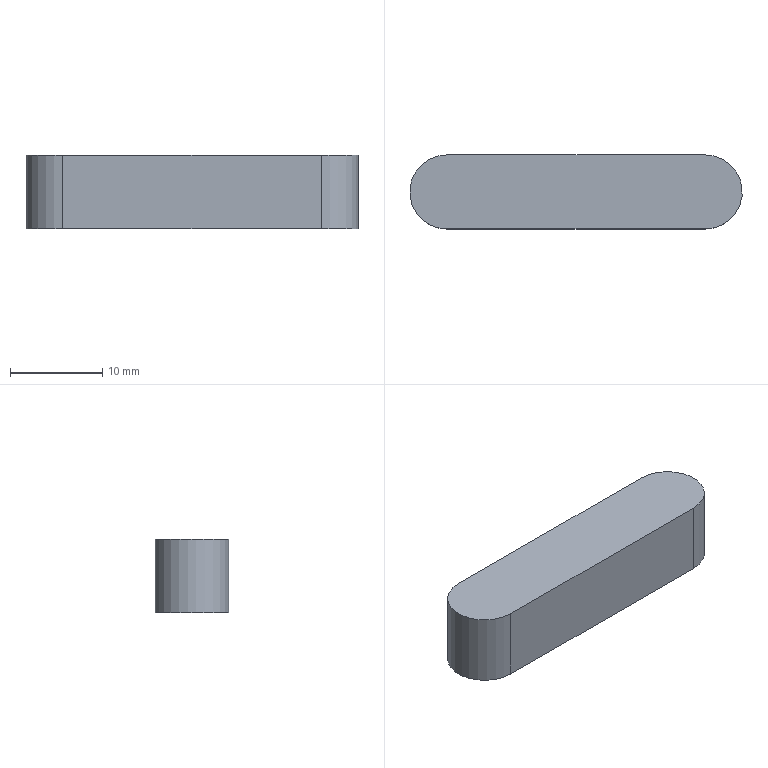Part | NX | features DATUM_CSYS 2, EXTRUDE 1, SKETCH 1 | 1 solid | 6 faces | box 36 x 8 x 8 mm | volume 2194 mm3 | plane 4 | cylinder 2 | commonest cylinder face diameters 8 x2
STEP:
#1=CARTESIAN_POINT('',(14.,-4.,0.));
#2=VERTEX_POINT('',#1);
#3=CARTESIAN_POINT('',(14.,4.,0.));
#4=VERTEX_POINT('',#3);
#5=CARTESIAN_POINT('',(14.,0.,0.));
#6=DIRECTION('',(0.,0.,1.));
#7=DIRECTION('',(-1.,0.,0.));
#8=AXIS2_PLACEMENT_3D('',#5,#6,#7);
#9=CIRCLE('',#8,4.);
#10=EDGE_CURVE('',#2,#4,#9,.T.);
#11=ORIENTED_EDGE('',*,*,#10,.T.);
#12=CARTESIAN_POINT('',(14.,4.,8.));
#13=VERTEX_POINT('',#12);
#14=CARTESIAN_POINT('',(14.,4.,8.));
#15=DIRECTION('',(0.,0.,-1.));
#16=VECTOR('',#15,1000.);
#17=LINE('',#14,#16);
#18=EDGE_CURVE('',#13,#4,#17,.T.);
#19=ORIENTED_EDGE('',*,*,#18,.F.);
#20=CARTESIAN_POINT('',(14.,-4.,8.));
#21=VERTEX_POINT('',#20);
#22=CARTESIAN_POINT('',(14.,0.,8.));
#23=DIRECTION('',(0.,0.,1.));
#24=DIRECTION('',(-1.,0.,0.));
#25=AXIS2_PLACEMENT_3D('',#22,#23,#24);
#26=CIRCLE('',#25,4.);
#27=EDGE_CURVE('',#21,#13,#26,.T.);
#28=ORIENTED_EDGE('',*,*,#27,.F.);
#29=CARTESIAN_POINT('',(14.,-4.,8.));
#30=DIRECTION('',(0.,0.,-1.));
#31=VECTOR('',#30,1000.);
#32=LINE('',#29,#31);
#33=EDGE_CURVE('',#21,#2,#32,.T.);
#34=ORIENTED_EDGE('',*,*,#33,.T.);
#35=EDGE_LOOP('',(#11,#19,#28,#34));
#36=FACE_BOUND('',#35,.T.);
#37=CARTESIAN_POINT('',(14.,0.,8.));
#38=DIRECTION('',(0.,0.,-1.));
#39=DIRECTION('',(-1.,0.,0.));
#40=AXIS2_PLACEMENT_3D('',#37,#38,#39);
#41=CYLINDRICAL_SURFACE('',#40,4.);
#42=ADVANCED_FACE('',(#36),#41,.T.);
#43=CARTESIAN_POINT('',(-14.,4.,0.));
#44=VERTEX_POINT('',#43);
#45=CARTESIAN_POINT('',(14.,4.,0.));
#46=DIRECTION('',(-1.,0.,0.));
#47=VECTOR('',#46,1000.);
#48=LINE('',#45,#47);
#49=EDGE_CURVE('',#4,#44,#48,.T.);
#50=ORIENTED_EDGE('',*,*,#49,.T.);
#51=CARTESIAN_POINT('',(-14.,4.,8.));
#52=VERTEX_POINT('',#51);
#53=CARTESIAN_POINT('',(-14.,4.,8.));
#54=DIRECTION('',(0.,0.,-1.));
#55=VECTOR('',#54,1000.);
#56=LINE('',#53,#55);
#57=EDGE_CURVE('',#52,#44,#56,.T.);
#58=ORIENTED_EDGE('',*,*,#57,.F.);
#59=CARTESIAN_POINT('',(14.,4.,8.));
#60=DIRECTION('',(-1.,0.,0.));
#61=VECTOR('',#60,1000.);
#62=LINE('',#59,#61);
#63=EDGE_CURVE('',#13,#52,#62,.T.);
#64=ORIENTED_EDGE('',*,*,#63,.F.);
#65=ORIENTED_EDGE('',*,*,#18,.T.);
#66=EDGE_LOOP('',(#50,#58,#64,#65));
#67=FACE_BOUND('',#66,.T.);
#68=CARTESIAN_POINT('',(14.,4.,8.));
#69=DIRECTION('',(0.,-1.,0.));
#70=DIRECTION('',(0.,0.,-1.));
#71=AXIS2_PLACEMENT_3D('',#68,#69,#70);
#72=PLANE('',#71);
#73=ADVANCED_FACE('',(#67),#72,.F.);
#74=CARTESIAN_POINT('',(-14.,-4.,0.));
#75=VERTEX_POINT('',#74);
#76=CARTESIAN_POINT('',(-14.,0.,0.));
#77=DIRECTION('',(0.,0.,1.));
#78=DIRECTION('',(1.,0.,0.));
#79=AXIS2_PLACEMENT_3D('',#76,#77,#78);
#80=CIRCLE('',#79,4.);
#81=EDGE_CURVE('',#44,#75,#80,.T.);
#82=ORIENTED_EDGE('',*,*,#81,.T.);
#83=CARTESIAN_POINT('',(-14.,-4.,8.));
#84=VERTEX_POINT('',#83);
#85=CARTESIAN_POINT('',(-14.,-4.,8.));
#86=DIRECTION('',(0.,0.,-1.));
#87=VECTOR('',#86,1000.);
#88=LINE('',#85,#87);
#89=EDGE_CURVE('',#84,#75,#88,.T.);
#90=ORIENTED_EDGE('',*,*,#89,.F.);
#91=CARTESIAN_POINT('',(-14.,0.,8.));
#92=DIRECTION('',(0.,0.,1.));
#93=DIRECTION('',(1.,0.,0.));
#94=AXIS2_PLACEMENT_3D('',#91,#92,#93);
#95=CIRCLE('',#94,4.);
#96=EDGE_CURVE('',#52,#84,#95,.T.);
#97=ORIENTED_EDGE('',*,*,#96,.F.);
#98=ORIENTED_EDGE('',*,*,#57,.T.);
#99=EDGE_LOOP('',(#82,#90,#97,#98));
#100=FACE_BOUND('',#99,.T.);
#101=CARTESIAN_POINT('',(-14.,0.,8.));
#102=DIRECTION('',(0.,0.,-1.));
#103=DIRECTION('',(-1.,0.,0.));
#104=AXIS2_PLACEMENT_3D('',#101,#102,#103);
#105=CYLINDRICAL_SURFACE('',#104,4.);
#106=ADVANCED_FACE('',(#100),#105,.T.);
#107=CARTESIAN_POINT('',(-14.,-4.,0.));
#108=DIRECTION('',(1.,0.,0.));
#109=VECTOR('',#108,1000.);
#110=LINE('',#107,#109);
#111=EDGE_CURVE('',#75,#2,#110,.T.);
#112=ORIENTED_EDGE('',*,*,#111,.T.);
#113=ORIENTED_EDGE('',*,*,#33,.F.);
#114=CARTESIAN_POINT('',(-14.,-4.,8.));
#115=DIRECTION('',(1.,0.,0.));
#116=VECTOR('',#115,1000.);
#117=LINE('',#114,#116);
#118=EDGE_CURVE('',#84,#21,#117,.T.);
#119=ORIENTED_EDGE('',*,*,#118,.F.);
#120=ORIENTED_EDGE('',*,*,#89,.T.);
#121=EDGE_LOOP('',(#112,#113,#119,#120));
#122=FACE_BOUND('',#121,.T.);
#123=CARTESIAN_POINT('',(-14.,-4.,8.));
#124=DIRECTION('',(0.,1.,0.));
#125=DIRECTION('',(0.,0.,1.));
#126=AXIS2_PLACEMENT_3D('',#123,#124,#125);
#127=PLANE('',#126);
#128=ADVANCED_FACE('',(#122),#127,.F.);
#129=ORIENTED_EDGE('',*,*,#27,.T.);
#130=ORIENTED_EDGE('',*,*,#63,.T.);
#131=ORIENTED_EDGE('',*,*,#96,.T.);
#132=ORIENTED_EDGE('',*,*,#118,.T.);
#133=EDGE_LOOP('',(#129,#130,#131,#132));
#134=FACE_BOUND('',#133,.T.);
#135=CARTESIAN_POINT('',(14.,0.,8.));
#136=DIRECTION('',(0.,0.,1.));
#137=DIRECTION('',(1.,0.,0.));
#138=AXIS2_PLACEMENT_3D('',#135,#136,#137);
#139=PLANE('',#138);
#140=ADVANCED_FACE('',(#134),#139,.T.);
#141=ORIENTED_EDGE('',*,*,#10,.F.);
#142=ORIENTED_EDGE('',*,*,#111,.F.);
#143=ORIENTED_EDGE('',*,*,#81,.F.);
#144=ORIENTED_EDGE('',*,*,#49,.F.);
#145=EDGE_LOOP('',(#141,#142,#143,#144));
#146=FACE_BOUND('',#145,.T.);
#147=CARTESIAN_POINT('',(14.,0.,0.));
#148=DIRECTION('',(0.,0.,1.));
#149=DIRECTION('',(1.,0.,0.));
#150=AXIS2_PLACEMENT_3D('',#147,#148,#149);
#151=PLANE('',#150);
#152=ADVANCED_FACE('',(#146),#151,.F.);
#153=CLOSED_SHELL('',(#42,#73,#106,#128,#140,#152));
#154=MANIFOLD_SOLID_BREP('',#153);
#155=(LENGTH_UNIT()NAMED_UNIT(*)SI_UNIT(.MILLI.,.METRE.));
#156=UNCERTAINTY_MEASURE_WITH_UNIT(LENGTH_MEASURE(0.00001),#155,'','');
#157=(NAMED_UNIT(*)PLANE_ANGLE_UNIT()SI_UNIT($,.RADIAN.));
#158=(NAMED_UNIT(*)SI_UNIT($,.STERADIAN.)SOLID_ANGLE_UNIT());
#159=(GEOMETRIC_REPRESENTATION_CONTEXT(3)GLOBAL_UNCERTAINTY_ASSIGNED_CONTEXT((#156))GLOBAL_UNIT_ASSIGNED_CONTEXT((#155,#157,#158))REPRESENTATION_CONTEXT('',''));
#160=ADVANCED_BREP_SHAPE_REPRESENTATION('',(#154),#159);